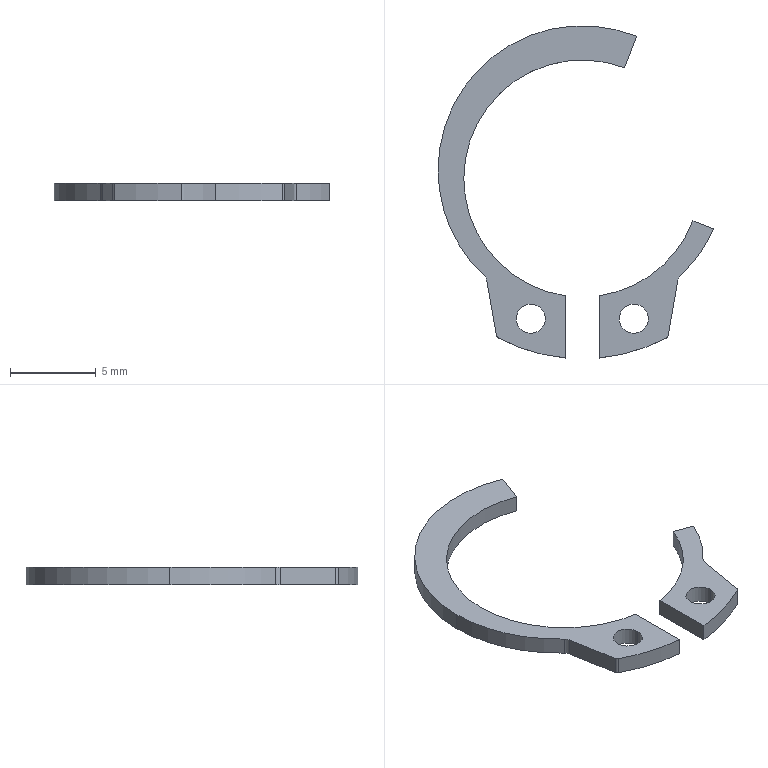Part | STEP file | Shaft retaining ring type A 15 | 2 solids | 26 faces | box 16.068 x 19.352 x 1 mm | volume 68.849 mm3 | cylinder 16 | plane 10 | commonest cylinder face diameters 1.7 x4 13.8 x3 16.8 x3 0.4 x2 1 x2 21 x2